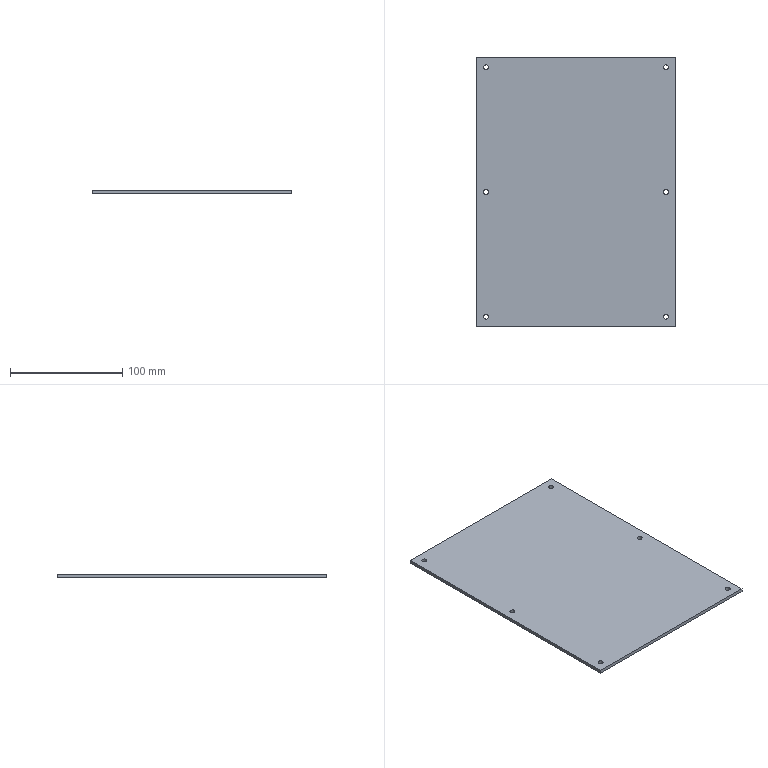Part | SolidWorks | features Cut 1, Extrusion 1 | 1 solid | 18 faces | box 178 x 240 x 3 mm | volume 127886 mm3 | cylinder 12 | plane 6 | commonest cylinder face diameters 4.4 x12
STEP:
#1=CARTESIAN_POINT('',(77.8,111.,0.));
#2=VERTEX_POINT('',#1);
#3=CARTESIAN_POINT('',(82.2,111.,0.));
#4=VERTEX_POINT('',#3);
#5=CARTESIAN_POINT('',(80.,111.,0.));
#6=DIRECTION('',(0.,0.,1.));
#7=DIRECTION('',(1.,0.,0.));
#8=AXIS2_PLACEMENT_3D('',#5,#6,#7);
#9=CIRCLE('',#8,2.2);
#10=EDGE_CURVE('',#2,#4,#9,.T.);
#11=ORIENTED_EDGE('',*,*,#10,.F.);
#12=CARTESIAN_POINT('',(77.8,111.,3.));
#13=VERTEX_POINT('',#12);
#14=CARTESIAN_POINT('',(77.8,111.,-7.));
#15=DIRECTION('',(0.,0.,1.));
#16=VECTOR('',#15,1000.);
#17=LINE('',#14,#16);
#18=EDGE_CURVE('',#2,#13,#17,.T.);
#19=ORIENTED_EDGE('',*,*,#18,.T.);
#20=CARTESIAN_POINT('',(82.2,111.,3.));
#21=VERTEX_POINT('',#20);
#22=CARTESIAN_POINT('',(80.,111.,3.));
#23=DIRECTION('',(0.,0.,1.));
#24=DIRECTION('',(1.,0.,0.));
#25=AXIS2_PLACEMENT_3D('',#22,#23,#24);
#26=CIRCLE('',#25,2.2);
#27=EDGE_CURVE('',#13,#21,#26,.T.);
#28=ORIENTED_EDGE('',*,*,#27,.T.);
#29=CARTESIAN_POINT('',(82.2,111.,-7.));
#30=DIRECTION('',(0.,0.,1.));
#31=VECTOR('',#30,1000.);
#32=LINE('',#29,#31);
#33=EDGE_CURVE('',#4,#21,#32,.T.);
#34=ORIENTED_EDGE('',*,*,#33,.F.);
#35=EDGE_LOOP('',(#11,#19,#28,#34));
#36=FACE_OUTER_BOUND('',#35,.T.);
#37=CARTESIAN_POINT('',(80.,111.,-7.));
#38=DIRECTION('',(0.,0.,1.));
#39=DIRECTION('',(1.,0.,0.));
#40=AXIS2_PLACEMENT_3D('',#37,#38,#39);
#41=CYLINDRICAL_SURFACE('',#40,2.2);
#42=ADVANCED_FACE('',(#36),#41,.F.);
#43=CARTESIAN_POINT('',(77.8,-111.,0.));
#44=VERTEX_POINT('',#43);
#45=CARTESIAN_POINT('',(82.2,-111.,0.));
#46=VERTEX_POINT('',#45);
#47=CARTESIAN_POINT('',(80.,-111.,0.));
#48=DIRECTION('',(0.,0.,1.));
#49=DIRECTION('',(1.,0.,0.));
#50=AXIS2_PLACEMENT_3D('',#47,#48,#49);
#51=CIRCLE('',#50,2.2);
#52=EDGE_CURVE('',#44,#46,#51,.T.);
#53=ORIENTED_EDGE('',*,*,#52,.F.);
#54=CARTESIAN_POINT('',(77.8,-111.,3.));
#55=VERTEX_POINT('',#54);
#56=CARTESIAN_POINT('',(77.8,-111.,-7.));
#57=DIRECTION('',(0.,0.,1.));
#58=VECTOR('',#57,1000.);
#59=LINE('',#56,#58);
#60=EDGE_CURVE('',#44,#55,#59,.T.);
#61=ORIENTED_EDGE('',*,*,#60,.T.);
#62=CARTESIAN_POINT('',(82.2,-111.,3.));
#63=VERTEX_POINT('',#62);
#64=CARTESIAN_POINT('',(80.,-111.,3.));
#65=DIRECTION('',(0.,0.,1.));
#66=DIRECTION('',(1.,0.,0.));
#67=AXIS2_PLACEMENT_3D('',#64,#65,#66);
#68=CIRCLE('',#67,2.2);
#69=EDGE_CURVE('',#55,#63,#68,.T.);
#70=ORIENTED_EDGE('',*,*,#69,.T.);
#71=CARTESIAN_POINT('',(82.2,-111.,-7.));
#72=DIRECTION('',(0.,0.,1.));
#73=VECTOR('',#72,1000.);
#74=LINE('',#71,#73);
#75=EDGE_CURVE('',#46,#63,#74,.T.);
#76=ORIENTED_EDGE('',*,*,#75,.F.);
#77=EDGE_LOOP('',(#53,#61,#70,#76));
#78=FACE_OUTER_BOUND('',#77,.T.);
#79=CARTESIAN_POINT('',(80.,-111.,-7.));
#80=DIRECTION('',(0.,0.,1.));
#81=DIRECTION('',(1.,0.,0.));
#82=AXIS2_PLACEMENT_3D('',#79,#80,#81);
#83=CYLINDRICAL_SURFACE('',#82,2.2);
#84=ADVANCED_FACE('',(#78),#83,.F.);
#85=CARTESIAN_POINT('',(-82.2,-111.,0.));
#86=VERTEX_POINT('',#85);
#87=CARTESIAN_POINT('',(-77.8,-111.,0.));
#88=VERTEX_POINT('',#87);
#89=CARTESIAN_POINT('',(-80.,-111.,0.));
#90=DIRECTION('',(0.,0.,1.));
#91=DIRECTION('',(1.,0.,0.));
#92=AXIS2_PLACEMENT_3D('',#89,#90,#91);
#93=CIRCLE('',#92,2.2);
#94=EDGE_CURVE('',#86,#88,#93,.T.);
#95=ORIENTED_EDGE('',*,*,#94,.F.);
#96=CARTESIAN_POINT('',(-82.2,-111.,3.));
#97=VERTEX_POINT('',#96);
#98=CARTESIAN_POINT('',(-82.2,-111.,-7.));
#99=DIRECTION('',(0.,0.,1.));
#100=VECTOR('',#99,1000.);
#101=LINE('',#98,#100);
#102=EDGE_CURVE('',#86,#97,#101,.T.);
#103=ORIENTED_EDGE('',*,*,#102,.T.);
#104=CARTESIAN_POINT('',(-77.8,-111.,3.));
#105=VERTEX_POINT('',#104);
#106=CARTESIAN_POINT('',(-80.,-111.,3.));
#107=DIRECTION('',(0.,0.,1.));
#108=DIRECTION('',(1.,0.,0.));
#109=AXIS2_PLACEMENT_3D('',#106,#107,#108);
#110=CIRCLE('',#109,2.2);
#111=EDGE_CURVE('',#97,#105,#110,.T.);
#112=ORIENTED_EDGE('',*,*,#111,.T.);
#113=CARTESIAN_POINT('',(-77.8,-111.,-7.));
#114=DIRECTION('',(0.,0.,1.));
#115=VECTOR('',#114,1000.);
#116=LINE('',#113,#115);
#117=EDGE_CURVE('',#88,#105,#116,.T.);
#118=ORIENTED_EDGE('',*,*,#117,.F.);
#119=EDGE_LOOP('',(#95,#103,#112,#118));
#120=FACE_OUTER_BOUND('',#119,.T.);
#121=CARTESIAN_POINT('',(-80.,-111.,-7.));
#122=DIRECTION('',(0.,0.,1.));
#123=DIRECTION('',(1.,0.,0.));
#124=AXIS2_PLACEMENT_3D('',#121,#122,#123);
#125=CYLINDRICAL_SURFACE('',#124,2.2);
#126=ADVANCED_FACE('',(#120),#125,.F.);
#127=CARTESIAN_POINT('',(-82.2,0.,0.));
#128=VERTEX_POINT('',#127);
#129=CARTESIAN_POINT('',(-77.8,0.,0.));
#130=VERTEX_POINT('',#129);
#131=CARTESIAN_POINT('',(-80.,0.,0.));
#132=DIRECTION('',(0.,0.,1.));
#133=DIRECTION('',(1.,0.,0.));
#134=AXIS2_PLACEMENT_3D('',#131,#132,#133);
#135=CIRCLE('',#134,2.2);
#136=EDGE_CURVE('',#128,#130,#135,.T.);
#137=ORIENTED_EDGE('',*,*,#136,.F.);
#138=CARTESIAN_POINT('',(-82.2,0.,3.));
#139=VERTEX_POINT('',#138);
#140=CARTESIAN_POINT('',(-82.2,0.,-7.));
#141=DIRECTION('',(0.,0.,1.));
#142=VECTOR('',#141,1000.);
#143=LINE('',#140,#142);
#144=EDGE_CURVE('',#128,#139,#143,.T.);
#145=ORIENTED_EDGE('',*,*,#144,.T.);
#146=CARTESIAN_POINT('',(-77.8,0.,3.));
#147=VERTEX_POINT('',#146);
#148=CARTESIAN_POINT('',(-80.,0.,3.));
#149=DIRECTION('',(0.,0.,1.));
#150=DIRECTION('',(1.,0.,0.));
#151=AXIS2_PLACEMENT_3D('',#148,#149,#150);
#152=CIRCLE('',#151,2.2);
#153=EDGE_CURVE('',#139,#147,#152,.T.);
#154=ORIENTED_EDGE('',*,*,#153,.T.);
#155=CARTESIAN_POINT('',(-77.8,0.,-7.));
#156=DIRECTION('',(0.,0.,1.));
#157=VECTOR('',#156,1000.);
#158=LINE('',#155,#157);
#159=EDGE_CURVE('',#130,#147,#158,.T.);
#160=ORIENTED_EDGE('',*,*,#159,.F.);
#161=EDGE_LOOP('',(#137,#145,#154,#160));
#162=FACE_OUTER_BOUND('',#161,.T.);
#163=CARTESIAN_POINT('',(-80.,0.,-7.));
#164=DIRECTION('',(0.,0.,1.));
#165=DIRECTION('',(1.,0.,0.));
#166=AXIS2_PLACEMENT_3D('',#163,#164,#165);
#167=CYLINDRICAL_SURFACE('',#166,2.2);
#168=ADVANCED_FACE('',(#162),#167,.F.);
#169=CARTESIAN_POINT('',(77.8,0.,0.));
#170=VERTEX_POINT('',#169);
#171=CARTESIAN_POINT('',(82.2,0.,0.));
#172=VERTEX_POINT('',#171);
#173=CARTESIAN_POINT('',(80.,0.,0.));
#174=DIRECTION('',(0.,0.,1.));
#175=DIRECTION('',(1.,0.,0.));
#176=AXIS2_PLACEMENT_3D('',#173,#174,#175);
#177=CIRCLE('',#176,2.2);
#178=EDGE_CURVE('',#170,#172,#177,.T.);
#179=ORIENTED_EDGE('',*,*,#178,.F.);
#180=CARTESIAN_POINT('',(77.8,0.,3.));
#181=VERTEX_POINT('',#180);
#182=CARTESIAN_POINT('',(77.8,0.,-7.));
#183=DIRECTION('',(0.,0.,1.));
#184=VECTOR('',#183,1000.);
#185=LINE('',#182,#184);
#186=EDGE_CURVE('',#170,#181,#185,.T.);
#187=ORIENTED_EDGE('',*,*,#186,.T.);
#188=CARTESIAN_POINT('',(82.2,0.,3.));
#189=VERTEX_POINT('',#188);
#190=CARTESIAN_POINT('',(80.,0.,3.));
#191=DIRECTION('',(0.,0.,1.));
#192=DIRECTION('',(1.,0.,0.));
#193=AXIS2_PLACEMENT_3D('',#190,#191,#192);
#194=CIRCLE('',#193,2.2);
#195=EDGE_CURVE('',#181,#189,#194,.T.);
#196=ORIENTED_EDGE('',*,*,#195,.T.);
#197=CARTESIAN_POINT('',(82.2,0.,-7.));
#198=DIRECTION('',(0.,0.,1.));
#199=VECTOR('',#198,1000.);
#200=LINE('',#197,#199);
#201=EDGE_CURVE('',#172,#189,#200,.T.);
#202=ORIENTED_EDGE('',*,*,#201,.F.);
#203=EDGE_LOOP('',(#179,#187,#196,#202));
#204=FACE_OUTER_BOUND('',#203,.T.);
#205=CARTESIAN_POINT('',(80.,0.,-7.));
#206=DIRECTION('',(0.,0.,1.));
#207=DIRECTION('',(1.,0.,0.));
#208=AXIS2_PLACEMENT_3D('',#205,#206,#207);
#209=CYLINDRICAL_SURFACE('',#208,2.2);
#210=ADVANCED_FACE('',(#204),#209,.F.);
#211=CARTESIAN_POINT('',(-82.2,111.,0.));
#212=VERTEX_POINT('',#211);
#213=CARTESIAN_POINT('',(-77.8,111.,0.));
#214=VERTEX_POINT('',#213);
#215=CARTESIAN_POINT('',(-80.,111.,0.));
#216=DIRECTION('',(0.,0.,1.));
#217=DIRECTION('',(1.,0.,0.));
#218=AXIS2_PLACEMENT_3D('',#215,#216,#217);
#219=CIRCLE('',#218,2.2);
#220=EDGE_CURVE('',#212,#214,#219,.T.);
#221=ORIENTED_EDGE('',*,*,#220,.F.);
#222=CARTESIAN_POINT('',(-82.2,111.,3.));
#223=VERTEX_POINT('',#222);
#224=CARTESIAN_POINT('',(-82.2,111.,-7.));
#225=DIRECTION('',(0.,0.,1.));
#226=VECTOR('',#225,1000.);
#227=LINE('',#224,#226);
#228=EDGE_CURVE('',#212,#223,#227,.T.);
#229=ORIENTED_EDGE('',*,*,#228,.T.);
#230=CARTESIAN_POINT('',(-77.8,111.,3.));
#231=VERTEX_POINT('',#230);
#232=CARTESIAN_POINT('',(-80.,111.,3.));
#233=DIRECTION('',(0.,0.,1.));
#234=DIRECTION('',(1.,0.,0.));
#235=AXIS2_PLACEMENT_3D('',#232,#233,#234);
#236=CIRCLE('',#235,2.2);
#237=EDGE_CURVE('',#223,#231,#236,.T.);
#238=ORIENTED_EDGE('',*,*,#237,.T.);
#239=CARTESIAN_POINT('',(-77.8,111.,-7.));
#240=DIRECTION('',(0.,0.,1.));
#241=VECTOR('',#240,1000.);
#242=LINE('',#239,#241);
#243=EDGE_CURVE('',#214,#231,#242,.T.);
#244=ORIENTED_EDGE('',*,*,#243,.F.);
#245=EDGE_LOOP('',(#221,#229,#238,#244));
#246=FACE_OUTER_BOUND('',#245,.T.);
#247=CARTESIAN_POINT('',(-80.,111.,-7.));
#248=DIRECTION('',(0.,0.,1.));
#249=DIRECTION('',(1.,0.,0.));
#250=AXIS2_PLACEMENT_3D('',#247,#248,#249);
#251=CYLINDRICAL_SURFACE('',#250,2.2);
#252=ADVANCED_FACE('',(#246),#251,.F.);
#253=CARTESIAN_POINT('',(-89.,120.,0.));
#254=VERTEX_POINT('',#253);
#255=CARTESIAN_POINT('',(-89.,-120.,0.));
#256=VERTEX_POINT('',#255);
#257=CARTESIAN_POINT('',(-89.,-120.,0.));
#258=DIRECTION('',(0.,-1.,0.));
#259=VECTOR('',#258,1000.);
#260=LINE('',#257,#259);
#261=EDGE_CURVE('',#254,#256,#260,.T.);
#262=ORIENTED_EDGE('',*,*,#261,.T.);
#263=CARTESIAN_POINT('',(-89.,-120.,3.));
#264=VERTEX_POINT('',#263);
#265=CARTESIAN_POINT('',(-89.,-120.,3.));
#266=DIRECTION('',(0.,0.,-1.));
#267=VECTOR('',#266,1000.);
#268=LINE('',#265,#267);
#269=EDGE_CURVE('',#264,#256,#268,.T.);
#270=ORIENTED_EDGE('',*,*,#269,.F.);
#271=CARTESIAN_POINT('',(-89.,120.,3.));
#272=VERTEX_POINT('',#271);
#273=CARTESIAN_POINT('',(-89.,-120.,3.));
#274=DIRECTION('',(0.,-1.,0.));
#275=VECTOR('',#274,1000.);
#276=LINE('',#273,#275);
#277=EDGE_CURVE('',#272,#264,#276,.T.);
#278=ORIENTED_EDGE('',*,*,#277,.F.);
#279=CARTESIAN_POINT('',(-89.,120.,3.));
#280=DIRECTION('',(0.,0.,-1.));
#281=VECTOR('',#280,1000.);
#282=LINE('',#279,#281);
#283=EDGE_CURVE('',#272,#254,#282,.T.);
#284=ORIENTED_EDGE('',*,*,#283,.T.);
#285=EDGE_LOOP('',(#262,#270,#278,#284));
#286=FACE_OUTER_BOUND('',#285,.T.);
#287=CARTESIAN_POINT('',(-89.,-120.,3.));
#288=DIRECTION('',(1.,0.,0.));
#289=DIRECTION('',(0.,0.,-1.));
#290=AXIS2_PLACEMENT_3D('',#287,#288,#289);
#291=PLANE('',#290);
#292=ADVANCED_FACE('',(#286),#291,.F.);
#293=CARTESIAN_POINT('',(89.,-120.,0.));
#294=VERTEX_POINT('',#293);
#295=CARTESIAN_POINT('',(89.,-120.,0.));
#296=DIRECTION('',(1.,0.,0.));
#297=VECTOR('',#296,1000.);
#298=LINE('',#295,#297);
#299=EDGE_CURVE('',#256,#294,#298,.T.);
#300=ORIENTED_EDGE('',*,*,#299,.T.);
#301=CARTESIAN_POINT('',(89.,-120.,3.));
#302=VERTEX_POINT('',#301);
#303=CARTESIAN_POINT('',(89.,-120.,3.));
#304=DIRECTION('',(0.,0.,-1.));
#305=VECTOR('',#304,1000.);
#306=LINE('',#303,#305);
#307=EDGE_CURVE('',#302,#294,#306,.T.);
#308=ORIENTED_EDGE('',*,*,#307,.F.);
#309=CARTESIAN_POINT('',(89.,-120.,3.));
#310=DIRECTION('',(1.,0.,0.));
#311=VECTOR('',#310,1000.);
#312=LINE('',#309,#311);
#313=EDGE_CURVE('',#264,#302,#312,.T.);
#314=ORIENTED_EDGE('',*,*,#313,.F.);
#315=ORIENTED_EDGE('',*,*,#269,.T.);
#316=EDGE_LOOP('',(#300,#308,#314,#315));
#317=FACE_OUTER_BOUND('',#316,.T.);
#318=CARTESIAN_POINT('',(89.,-120.,3.));
#319=DIRECTION('',(0.,1.,0.));
#320=DIRECTION('',(-1.,0.,0.));
#321=AXIS2_PLACEMENT_3D('',#318,#319,#320);
#322=PLANE('',#321);
#323=ADVANCED_FACE('',(#317),#322,.F.);
#324=CARTESIAN_POINT('',(89.,120.,0.));
#325=VERTEX_POINT('',#324);
#326=CARTESIAN_POINT('',(89.,-120.,0.));
#327=DIRECTION('',(0.,1.,0.));
#328=VECTOR('',#327,1000.);
#329=LINE('',#326,#328);
#330=EDGE_CURVE('',#294,#325,#329,.T.);
#331=ORIENTED_EDGE('',*,*,#330,.T.);
#332=CARTESIAN_POINT('',(89.,120.,3.));
#333=VERTEX_POINT('',#332);
#334=CARTESIAN_POINT('',(89.,120.,3.));
#335=DIRECTION('',(0.,0.,-1.));
#336=VECTOR('',#335,1000.);
#337=LINE('',#334,#336);
#338=EDGE_CURVE('',#333,#325,#337,.T.);
#339=ORIENTED_EDGE('',*,*,#338,.F.);
#340=CARTESIAN_POINT('',(89.,-120.,3.));
#341=DIRECTION('',(0.,1.,0.));
#342=VECTOR('',#341,1000.);
#343=LINE('',#340,#342);
#344=EDGE_CURVE('',#302,#333,#343,.T.);
#345=ORIENTED_EDGE('',*,*,#344,.F.);
#346=ORIENTED_EDGE('',*,*,#307,.T.);
#347=EDGE_LOOP('',(#331,#339,#345,#346));
#348=FACE_OUTER_BOUND('',#347,.T.);
#349=CARTESIAN_POINT('',(89.,-120.,3.));
#350=DIRECTION('',(-1.,0.,0.));
#351=DIRECTION('',(0.,0.,1.));
#352=AXIS2_PLACEMENT_3D('',#349,#350,#351);
#353=PLANE('',#352);
#354=ADVANCED_FACE('',(#348),#353,.F.);
#355=CARTESIAN_POINT('',(89.,120.,0.));
#356=DIRECTION('',(-1.,0.,0.));
#357=VECTOR('',#356,1000.);
#358=LINE('',#355,#357);
#359=EDGE_CURVE('',#325,#254,#358,.T.);
#360=ORIENTED_EDGE('',*,*,#359,.T.);
#361=ORIENTED_EDGE('',*,*,#283,.F.);
#362=CARTESIAN_POINT('',(89.,120.,3.));
#363=DIRECTION('',(-1.,0.,0.));
#364=VECTOR('',#363,1000.);
#365=LINE('',#362,#364);
#366=EDGE_CURVE('',#333,#272,#365,.T.);
#367=ORIENTED_EDGE('',*,*,#366,.F.);
#368=ORIENTED_EDGE('',*,*,#338,.T.);
#369=EDGE_LOOP('',(#360,#361,#367,#368));
#370=FACE_OUTER_BOUND('',#369,.T.);
#371=CARTESIAN_POINT('',(89.,120.,3.));
#372=DIRECTION('',(0.,-1.,0.));
#373=DIRECTION('',(1.,0.,0.));
#374=AXIS2_PLACEMENT_3D('',#371,#372,#373);
#375=PLANE('',#374);
#376=ADVANCED_FACE('',(#370),#375,.F.);
#377=CARTESIAN_POINT('',(80.,111.,3.));
#378=DIRECTION('',(0.,0.,1.));
#379=DIRECTION('',(1.,0.,0.));
#380=AXIS2_PLACEMENT_3D('',#377,#378,#379);
#381=CIRCLE('',#380,2.2);
#382=EDGE_CURVE('',#21,#13,#381,.T.);
#383=ORIENTED_EDGE('',*,*,#382,.F.);
#384=ORIENTED_EDGE('',*,*,#27,.F.);
#385=EDGE_LOOP('',(#383,#384));
#386=FACE_BOUND('',#385,.T.);
#387=CARTESIAN_POINT('',(80.,-111.,3.));
#388=DIRECTION('',(0.,0.,1.));
#389=DIRECTION('',(1.,0.,0.));
#390=AXIS2_PLACEMENT_3D('',#387,#388,#389);
#391=CIRCLE('',#390,2.2);
#392=EDGE_CURVE('',#63,#55,#391,.T.);
#393=ORIENTED_EDGE('',*,*,#392,.F.);
#394=ORIENTED_EDGE('',*,*,#69,.F.);
#395=EDGE_LOOP('',(#393,#394));
#396=FACE_BOUND('',#395,.T.);
#397=CARTESIAN_POINT('',(-80.,-111.,3.));
#398=DIRECTION('',(0.,0.,1.));
#399=DIRECTION('',(1.,0.,0.));
#400=AXIS2_PLACEMENT_3D('',#397,#398,#399);
#401=CIRCLE('',#400,2.2);
#402=EDGE_CURVE('',#105,#97,#401,.T.);
#403=ORIENTED_EDGE('',*,*,#402,.F.);
#404=ORIENTED_EDGE('',*,*,#111,.F.);
#405=EDGE_LOOP('',(#403,#404));
#406=FACE_BOUND('',#405,.T.);
#407=CARTESIAN_POINT('',(-80.,0.,3.));
#408=DIRECTION('',(0.,0.,1.));
#409=DIRECTION('',(1.,0.,0.));
#410=AXIS2_PLACEMENT_3D('',#407,#408,#409);
#411=CIRCLE('',#410,2.2);
#412=EDGE_CURVE('',#147,#139,#411,.T.);
#413=ORIENTED_EDGE('',*,*,#412,.F.);
#414=ORIENTED_EDGE('',*,*,#153,.F.);
#415=EDGE_LOOP('',(#413,#414));
#416=FACE_BOUND('',#415,.T.);
#417=CARTESIAN_POINT('',(80.,0.,3.));
#418=DIRECTION('',(0.,0.,1.));
#419=DIRECTION('',(1.,0.,0.));
#420=AXIS2_PLACEMENT_3D('',#417,#418,#419);
#421=CIRCLE('',#420,2.2);
#422=EDGE_CURVE('',#189,#181,#421,.T.);
#423=ORIENTED_EDGE('',*,*,#422,.F.);
#424=ORIENTED_EDGE('',*,*,#195,.F.);
#425=EDGE_LOOP('',(#423,#424));
#426=FACE_BOUND('',#425,.T.);
#427=CARTESIAN_POINT('',(-80.,111.,3.));
#428=DIRECTION('',(0.,0.,1.));
#429=DIRECTION('',(1.,0.,0.));
#430=AXIS2_PLACEMENT_3D('',#427,#428,#429);
#431=CIRCLE('',#430,2.2);
#432=EDGE_CURVE('',#231,#223,#431,.T.);
#433=ORIENTED_EDGE('',*,*,#432,.F.);
#434=ORIENTED_EDGE('',*,*,#237,.F.);
#435=EDGE_LOOP('',(#433,#434));
#436=FACE_BOUND('',#435,.T.);
#437=ORIENTED_EDGE('',*,*,#277,.T.);
#438=ORIENTED_EDGE('',*,*,#313,.T.);
#439=ORIENTED_EDGE('',*,*,#344,.T.);
#440=ORIENTED_EDGE('',*,*,#366,.T.);
#441=EDGE_LOOP('',(#437,#438,#439,#440));
#442=FACE_OUTER_BOUND('',#441,.T.);
#443=CARTESIAN_POINT('',(0.,0.,3.));
#444=DIRECTION('',(0.,0.,1.));
#445=DIRECTION('',(1.,0.,0.));
#446=AXIS2_PLACEMENT_3D('',#443,#444,#445);
#447=PLANE('',#446);
#448=ADVANCED_FACE('',(#386,#396,#406,#416,#426,#436,#442),#447,.T.);
#449=CARTESIAN_POINT('',(80.,111.,0.));
#450=DIRECTION('',(0.,0.,1.));
#451=DIRECTION('',(1.,0.,0.));
#452=AXIS2_PLACEMENT_3D('',#449,#450,#451);
#453=CIRCLE('',#452,2.2);
#454=EDGE_CURVE('',#4,#2,#453,.T.);
#455=ORIENTED_EDGE('',*,*,#454,.T.);
#456=ORIENTED_EDGE('',*,*,#10,.T.);
#457=EDGE_LOOP('',(#455,#456));
#458=FACE_BOUND('',#457,.T.);
#459=CARTESIAN_POINT('',(80.,-111.,0.));
#460=DIRECTION('',(0.,0.,1.));
#461=DIRECTION('',(1.,0.,0.));
#462=AXIS2_PLACEMENT_3D('',#459,#460,#461);
#463=CIRCLE('',#462,2.2);
#464=EDGE_CURVE('',#46,#44,#463,.T.);
#465=ORIENTED_EDGE('',*,*,#464,.T.);
#466=ORIENTED_EDGE('',*,*,#52,.T.);
#467=EDGE_LOOP('',(#465,#466));
#468=FACE_BOUND('',#467,.T.);
#469=CARTESIAN_POINT('',(-80.,-111.,0.));
#470=DIRECTION('',(0.,0.,1.));
#471=DIRECTION('',(1.,0.,0.));
#472=AXIS2_PLACEMENT_3D('',#469,#470,#471);
#473=CIRCLE('',#472,2.2);
#474=EDGE_CURVE('',#88,#86,#473,.T.);
#475=ORIENTED_EDGE('',*,*,#474,.T.);
#476=ORIENTED_EDGE('',*,*,#94,.T.);
#477=EDGE_LOOP('',(#475,#476));
#478=FACE_BOUND('',#477,.T.);
#479=CARTESIAN_POINT('',(-80.,0.,0.));
#480=DIRECTION('',(0.,0.,1.));
#481=DIRECTION('',(1.,0.,0.));
#482=AXIS2_PLACEMENT_3D('',#479,#480,#481);
#483=CIRCLE('',#482,2.2);
#484=EDGE_CURVE('',#130,#128,#483,.T.);
#485=ORIENTED_EDGE('',*,*,#484,.T.);
#486=ORIENTED_EDGE('',*,*,#136,.T.);
#487=EDGE_LOOP('',(#485,#486));
#488=FACE_BOUND('',#487,.T.);
#489=CARTESIAN_POINT('',(80.,0.,0.));
#490=DIRECTION('',(0.,0.,1.));
#491=DIRECTION('',(1.,0.,0.));
#492=AXIS2_PLACEMENT_3D('',#489,#490,#491);
#493=CIRCLE('',#492,2.2);
#494=EDGE_CURVE('',#172,#170,#493,.T.);
#495=ORIENTED_EDGE('',*,*,#494,.T.);
#496=ORIENTED_EDGE('',*,*,#178,.T.);
#497=EDGE_LOOP('',(#495,#496));
#498=FACE_BOUND('',#497,.T.);
#499=CARTESIAN_POINT('',(-80.,111.,0.));
#500=DIRECTION('',(0.,0.,1.));
#501=DIRECTION('',(1.,0.,0.));
#502=AXIS2_PLACEMENT_3D('',#499,#500,#501);
#503=CIRCLE('',#502,2.2);
#504=EDGE_CURVE('',#214,#212,#503,.T.);
#505=ORIENTED_EDGE('',*,*,#504,.T.);
#506=ORIENTED_EDGE('',*,*,#220,.T.);
#507=EDGE_LOOP('',(#505,#506));
#508=FACE_BOUND('',#507,.T.);
#509=ORIENTED_EDGE('',*,*,#261,.F.);
#510=ORIENTED_EDGE('',*,*,#359,.F.);
#511=ORIENTED_EDGE('',*,*,#330,.F.);
#512=ORIENTED_EDGE('',*,*,#299,.F.);
#513=EDGE_LOOP('',(#509,#510,#511,#512));
#514=FACE_OUTER_BOUND('',#513,.T.);
#515=CARTESIAN_POINT('',(0.,0.,0.));
#516=DIRECTION('',(0.,0.,1.));
#517=DIRECTION('',(1.,0.,0.));
#518=AXIS2_PLACEMENT_3D('',#515,#516,#517);
#519=PLANE('',#518);
#520=ADVANCED_FACE('',(#458,#468,#478,#488,#498,#508,#514),#519,.F.);
#521=ORIENTED_EDGE('',*,*,#228,.F.);
#522=ORIENTED_EDGE('',*,*,#504,.F.);
#523=ORIENTED_EDGE('',*,*,#243,.T.);
#524=ORIENTED_EDGE('',*,*,#432,.T.);
#525=EDGE_LOOP('',(#521,#522,#523,#524));
#526=FACE_OUTER_BOUND('',#525,.T.);
#527=CARTESIAN_POINT('',(-80.,111.,-7.));
#528=DIRECTION('',(0.,0.,1.));
#529=DIRECTION('',(1.,0.,0.));
#530=AXIS2_PLACEMENT_3D('',#527,#528,#529);
#531=CYLINDRICAL_SURFACE('',#530,2.2);
#532=ADVANCED_FACE('',(#526),#531,.F.);
#533=ORIENTED_EDGE('',*,*,#186,.F.);
#534=ORIENTED_EDGE('',*,*,#494,.F.);
#535=ORIENTED_EDGE('',*,*,#201,.T.);
#536=ORIENTED_EDGE('',*,*,#422,.T.);
#537=EDGE_LOOP('',(#533,#534,#535,#536));
#538=FACE_OUTER_BOUND('',#537,.T.);
#539=CARTESIAN_POINT('',(80.,0.,-7.));
#540=DIRECTION('',(0.,0.,1.));
#541=DIRECTION('',(1.,0.,0.));
#542=AXIS2_PLACEMENT_3D('',#539,#540,#541);
#543=CYLINDRICAL_SURFACE('',#542,2.2);
#544=ADVANCED_FACE('',(#538),#543,.F.);
#545=ORIENTED_EDGE('',*,*,#144,.F.);
#546=ORIENTED_EDGE('',*,*,#484,.F.);
#547=ORIENTED_EDGE('',*,*,#159,.T.);
#548=ORIENTED_EDGE('',*,*,#412,.T.);
#549=EDGE_LOOP('',(#545,#546,#547,#548));
#550=FACE_OUTER_BOUND('',#549,.T.);
#551=CARTESIAN_POINT('',(-80.,0.,-7.));
#552=DIRECTION('',(0.,0.,1.));
#553=DIRECTION('',(1.,0.,0.));
#554=AXIS2_PLACEMENT_3D('',#551,#552,#553);
#555=CYLINDRICAL_SURFACE('',#554,2.2);
#556=ADVANCED_FACE('',(#550),#555,.F.);
#557=ORIENTED_EDGE('',*,*,#102,.F.);
#558=ORIENTED_EDGE('',*,*,#474,.F.);
#559=ORIENTED_EDGE('',*,*,#117,.T.);
#560=ORIENTED_EDGE('',*,*,#402,.T.);
#561=EDGE_LOOP('',(#557,#558,#559,#560));
#562=FACE_OUTER_BOUND('',#561,.T.);
#563=CARTESIAN_POINT('',(-80.,-111.,-7.));
#564=DIRECTION('',(0.,0.,1.));
#565=DIRECTION('',(1.,0.,0.));
#566=AXIS2_PLACEMENT_3D('',#563,#564,#565);
#567=CYLINDRICAL_SURFACE('',#566,2.2);
#568=ADVANCED_FACE('',(#562),#567,.F.);
#569=ORIENTED_EDGE('',*,*,#60,.F.);
#570=ORIENTED_EDGE('',*,*,#464,.F.);
#571=ORIENTED_EDGE('',*,*,#75,.T.);
#572=ORIENTED_EDGE('',*,*,#392,.T.);
#573=EDGE_LOOP('',(#569,#570,#571,#572));
#574=FACE_OUTER_BOUND('',#573,.T.);
#575=CARTESIAN_POINT('',(80.,-111.,-7.));
#576=DIRECTION('',(0.,0.,1.));
#577=DIRECTION('',(1.,0.,0.));
#578=AXIS2_PLACEMENT_3D('',#575,#576,#577);
#579=CYLINDRICAL_SURFACE('',#578,2.2);
#580=ADVANCED_FACE('',(#574),#579,.F.);
#581=ORIENTED_EDGE('',*,*,#18,.F.);
#582=ORIENTED_EDGE('',*,*,#454,.F.);
#583=ORIENTED_EDGE('',*,*,#33,.T.);
#584=ORIENTED_EDGE('',*,*,#382,.T.);
#585=EDGE_LOOP('',(#581,#582,#583,#584));
#586=FACE_OUTER_BOUND('',#585,.T.);
#587=CARTESIAN_POINT('',(80.,111.,-7.));
#588=DIRECTION('',(0.,0.,1.));
#589=DIRECTION('',(1.,0.,0.));
#590=AXIS2_PLACEMENT_3D('',#587,#588,#589);
#591=CYLINDRICAL_SURFACE('',#590,2.2);
#592=ADVANCED_FACE('',(#586),#591,.F.);
#593=CLOSED_SHELL('',(#42,#84,#126,#168,#210,#252,#292,#323,#354,#376,#448,#520,#532,#544,#556,#568,#580,#592));
#594=MANIFOLD_SOLID_BREP('',#593);
#595=CARTESIAN_POINT('',(0.,0.,0.));
#596=DIRECTION('',(0.,0.,1.));
#597=DIRECTION('',(1.,0.,0.));
#598=AXIS2_PLACEMENT_3D('',#595,#596,#597);
#599=(LENGTH_UNIT()NAMED_UNIT(*)SI_UNIT(.MILLI.,.METRE.));
#600=UNCERTAINTY_MEASURE_WITH_UNIT(LENGTH_MEASURE(0.00001),#599,'','');
#601=(NAMED_UNIT(*)PLANE_ANGLE_UNIT()SI_UNIT($,.RADIAN.));
#602=(NAMED_UNIT(*)SI_UNIT($,.STERADIAN.)SOLID_ANGLE_UNIT());
#603=(GEOMETRIC_REPRESENTATION_CONTEXT(3)GLOBAL_UNCERTAINTY_ASSIGNED_CONTEXT((#600))GLOBAL_UNIT_ASSIGNED_CONTEXT((#599,#601,#602))REPRESENTATION_CONTEXT('',''));
#604=ADVANCED_BREP_SHAPE_REPRESENTATION('',(#594,#598),#603);